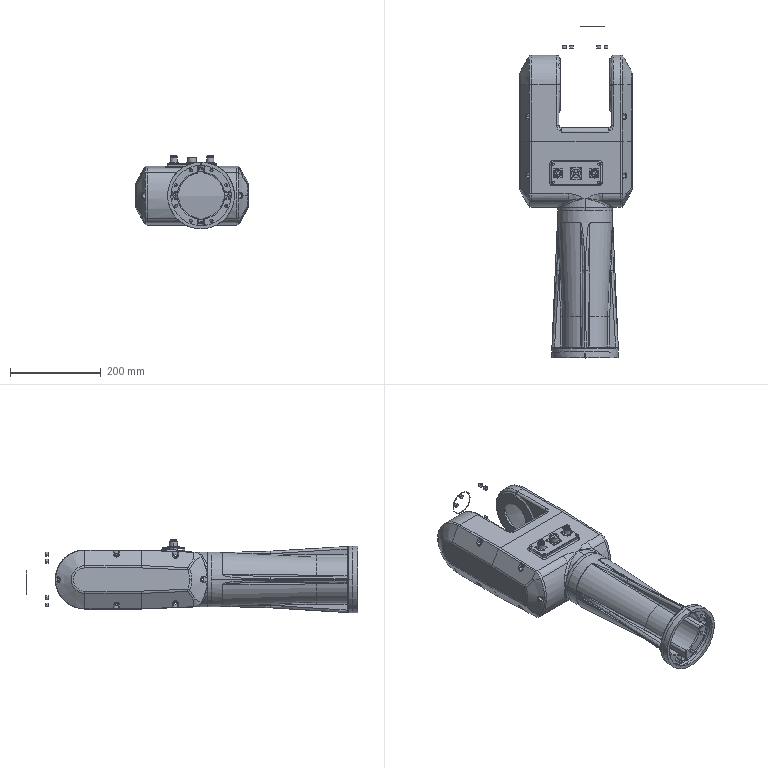Part | NX | features BREP 20 | 1 solid | 426 faces | box 247 x 731.027 x 162.5 mm | volume 8897535 mm3 | cylinder 164 | plane 98 | spline 79 | torus 56 | cone 26 | sphere 3 | commonest cylinder face diameters 4 x28 10 x19 7 x16 8.5 x16 9 x15 20 x11